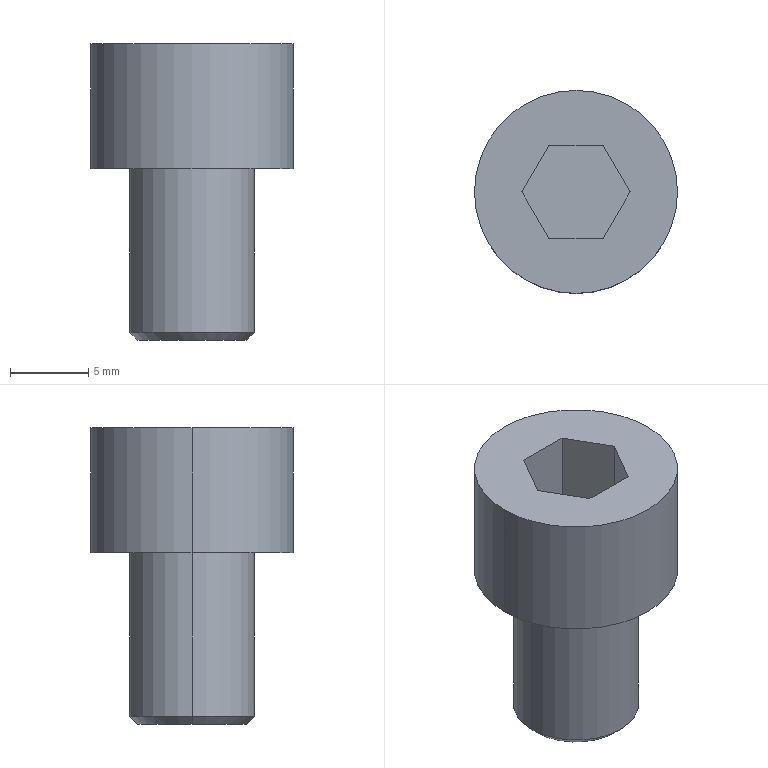Part | Creo | 1 solid | 16 faces | box 13 x 13 x 19 mm | volume 1447 mm3 | plane 10 | cylinder 4 | cone 2 | commonest cylinder face diameters 8 x2 13 x2
STEP:
#1=CARTESIAN_POINT('',(0.,0.,0.));
#2=DIRECTION('',(0.,0.,1.));
#3=DIRECTION('',(1.,0.,0.));
#4=AXIS2_PLACEMENT_3D('',#1,#2,#3);
#5=CARTESIAN_POINT('',(372.601,232.373,-47.934));
#6=VERTEX_POINT('',#5);
#7=CARTESIAN_POINT('',(380.601,232.373,-47.934));
#8=VERTEX_POINT('',#7);
#9=CARTESIAN_POINT('',(376.601,232.373,-47.934));
#10=DIRECTION('',(0.,0.,-1.));
#11=DIRECTION('',(-1.,0.,0.));
#12=AXIS2_PLACEMENT_3D('',#9,#10,#11);
#13=CIRCLE('',#12,4.);
#14=EDGE_CURVE('',#6,#8,#13,.T.);
#15=ORIENTED_EDGE('',*,*,#14,.T.);
#16=CARTESIAN_POINT('',(380.601,232.373,-37.441));
#17=VERTEX_POINT('',#16);
#18=CARTESIAN_POINT('',(380.601,232.373,-37.441));
#19=DIRECTION('',(0.,0.,-1.));
#20=VECTOR('',#19,10.493);
#21=LINE('',#18,#20);
#22=EDGE_CURVE('',#17,#8,#21,.T.);
#23=ORIENTED_EDGE('',*,*,#22,.F.);
#24=CARTESIAN_POINT('',(372.601,232.373,-37.441));
#25=VERTEX_POINT('',#24);
#26=CARTESIAN_POINT('',(376.601,232.373,-37.441));
#27=DIRECTION('',(0.,0.,1.));
#28=DIRECTION('',(1.,0.,0.));
#29=AXIS2_PLACEMENT_3D('',#26,#27,#28);
#30=CIRCLE('',#29,4.);
#31=EDGE_CURVE('',#17,#25,#30,.T.);
#32=ORIENTED_EDGE('',*,*,#31,.T.);
#33=CARTESIAN_POINT('',(372.601,232.373,-37.441));
#34=DIRECTION('',(0.,0.,-1.));
#35=VECTOR('',#34,10.493);
#36=LINE('',#33,#35);
#37=EDGE_CURVE('',#25,#6,#36,.T.);
#38=ORIENTED_EDGE('',*,*,#37,.T.);
#39=EDGE_LOOP('',(#15,#23,#32,#38));
#40=FACE_OUTER_BOUND('',#39,.F.);
#41=CARTESIAN_POINT('',(376.601,232.373,-37.441));
#42=DIRECTION('',(0.,0.,-1.));
#43=DIRECTION('',(-1.,0.,0.));
#44=AXIS2_PLACEMENT_3D('',#41,#42,#43);
#45=CYLINDRICAL_SURFACE('',#44,4.);
#46=ADVANCED_FACE('',(#40),#45,.T.);
#47=CARTESIAN_POINT('',(373.108,232.373,-48.441));
#48=VERTEX_POINT('',#47);
#49=CARTESIAN_POINT('',(380.093,232.373,-48.441));
#50=VERTEX_POINT('',#49);
#51=CARTESIAN_POINT('',(376.601,232.373,-48.441));
#52=DIRECTION('',(0.,0.,-1.));
#53=DIRECTION('',(-1.,0.,0.));
#54=AXIS2_PLACEMENT_3D('',#51,#52,#53);
#55=CIRCLE('',#54,3.493);
#56=EDGE_CURVE('',#48,#50,#55,.T.);
#57=ORIENTED_EDGE('',*,*,#56,.T.);
#58=CARTESIAN_POINT('',(380.093,232.373,-48.441));
#59=DIRECTION('',(0.7071,0.,0.7071));
#60=VECTOR('',#59,0.7176);
#61=LINE('',#58,#60);
#62=EDGE_CURVE('',#50,#8,#61,.T.);
#63=ORIENTED_EDGE('',*,*,#62,.T.);
#64=ORIENTED_EDGE('',*,*,#14,.F.);
#65=CARTESIAN_POINT('',(373.108,232.373,-48.441));
#66=DIRECTION('',(-0.7071,0.,0.7071));
#67=VECTOR('',#66,0.7176);
#68=LINE('',#65,#67);
#69=EDGE_CURVE('',#48,#6,#68,.T.);
#70=ORIENTED_EDGE('',*,*,#69,.F.);
#71=EDGE_LOOP('',(#57,#63,#64,#70));
#72=FACE_OUTER_BOUND('',#71,.F.);
#73=CARTESIAN_POINT('',(376.601,232.373,-48.188));
#74=DIRECTION('',(0.,0.,1.));
#75=DIRECTION('',(1.,0.,0.));
#76=AXIS2_PLACEMENT_3D('',#73,#74,#75);
#77=CONICAL_SURFACE('',#76,3.746,45.);
#78=ADVANCED_FACE('',(#72),#77,.T.);
#79=ORIENTED_EDGE('',*,*,#56,.F.);
#80=CARTESIAN_POINT('',(376.601,232.373,-48.441));
#81=DIRECTION('',(0.,0.,-1.));
#82=DIRECTION('',(1.,0.,0.));
#83=AXIS2_PLACEMENT_3D('',#80,#81,#82);
#84=CIRCLE('',#83,3.493);
#85=EDGE_CURVE('',#50,#48,#84,.T.);
#86=ORIENTED_EDGE('',*,*,#85,.F.);
#87=EDGE_LOOP('',(#79,#86));
#88=FACE_OUTER_BOUND('',#87,.F.);
#89=CARTESIAN_POINT('',(376.601,232.373,-48.441));
#90=DIRECTION('',(0.,0.,1.));
#91=DIRECTION('',(1.,0.,0.));
#92=AXIS2_PLACEMENT_3D('',#89,#90,#91);
#93=PLANE('',#92);
#94=ADVANCED_FACE('',(#88),#93,.F.);
#95=ORIENTED_EDGE('',*,*,#85,.T.);
#96=ORIENTED_EDGE('',*,*,#69,.T.);
#97=CARTESIAN_POINT('',(376.601,232.373,-47.934));
#98=DIRECTION('',(0.,0.,-1.));
#99=DIRECTION('',(1.,0.,0.));
#100=AXIS2_PLACEMENT_3D('',#97,#98,#99);
#101=CIRCLE('',#100,4.);
#102=EDGE_CURVE('',#8,#6,#101,.T.);
#103=ORIENTED_EDGE('',*,*,#102,.F.);
#104=ORIENTED_EDGE('',*,*,#62,.F.);
#105=EDGE_LOOP('',(#95,#96,#103,#104));
#106=FACE_OUTER_BOUND('',#105,.F.);
#107=CARTESIAN_POINT('',(376.601,232.373,-48.188));
#108=DIRECTION('',(0.,0.,1.));
#109=DIRECTION('',(1.,0.,0.));
#110=AXIS2_PLACEMENT_3D('',#107,#108,#109);
#111=CONICAL_SURFACE('',#110,3.746,45.);
#112=ADVANCED_FACE('',(#106),#111,.T.);
#113=ORIENTED_EDGE('',*,*,#102,.T.);
#114=ORIENTED_EDGE('',*,*,#37,.F.);
#115=CARTESIAN_POINT('',(376.601,232.373,-37.441));
#116=DIRECTION('',(0.,0.,1.));
#117=DIRECTION('',(-1.,0.,0.));
#118=AXIS2_PLACEMENT_3D('',#115,#116,#117);
#119=CIRCLE('',#118,4.);
#120=EDGE_CURVE('',#25,#17,#119,.T.);
#121=ORIENTED_EDGE('',*,*,#120,.T.);
#122=ORIENTED_EDGE('',*,*,#22,.T.);
#123=EDGE_LOOP('',(#113,#114,#121,#122));
#124=FACE_OUTER_BOUND('',#123,.F.);
#125=CARTESIAN_POINT('',(376.601,232.373,-37.441));
#126=DIRECTION('',(0.,0.,-1.));
#127=DIRECTION('',(-1.,0.,0.));
#128=AXIS2_PLACEMENT_3D('',#125,#126,#127);
#129=CYLINDRICAL_SURFACE('',#128,4.);
#130=ADVANCED_FACE('',(#124),#129,.T.);
#131=CARTESIAN_POINT('',(370.101,232.373,-37.441));
#132=VERTEX_POINT('',#131);
#133=CARTESIAN_POINT('',(383.101,232.373,-37.441));
#134=VERTEX_POINT('',#133);
#135=CARTESIAN_POINT('',(376.601,232.373,-37.441));
#136=DIRECTION('',(0.,0.,-1.));
#137=DIRECTION('',(-1.,0.,0.));
#138=AXIS2_PLACEMENT_3D('',#135,#136,#137);
#139=CIRCLE('',#138,6.5);
#140=EDGE_CURVE('',#132,#134,#139,.T.);
#141=ORIENTED_EDGE('',*,*,#140,.F.);
#142=CARTESIAN_POINT('',(376.601,232.373,-37.441));
#143=DIRECTION('',(0.,0.,-1.));
#144=DIRECTION('',(1.,0.,0.));
#145=AXIS2_PLACEMENT_3D('',#142,#143,#144);
#146=CIRCLE('',#145,6.5);
#147=EDGE_CURVE('',#134,#132,#146,.T.);
#148=ORIENTED_EDGE('',*,*,#147,.F.);
#149=EDGE_LOOP('',(#141,#148));
#150=FACE_OUTER_BOUND('',#149,.F.);
#151=ORIENTED_EDGE('',*,*,#120,.F.);
#152=ORIENTED_EDGE('',*,*,#31,.F.);
#153=EDGE_LOOP('',(#151,#152));
#154=FACE_BOUND('',#153,.F.);
#155=CARTESIAN_POINT('',(376.601,232.373,-37.441));
#156=DIRECTION('',(0.,0.,-1.));
#157=DIRECTION('',(-1.,0.,0.));
#158=AXIS2_PLACEMENT_3D('',#155,#156,#157);
#159=PLANE('',#158);
#160=ADVANCED_FACE('',(#150,#154),#159,.T.);
#161=CARTESIAN_POINT('',(383.101,232.373,-29.441));
#162=VERTEX_POINT('',#161);
#163=CARTESIAN_POINT('',(370.101,232.373,-29.441));
#164=VERTEX_POINT('',#163);
#165=CARTESIAN_POINT('',(376.601,232.373,-29.441));
#166=DIRECTION('',(0.,0.,1.));
#167=DIRECTION('',(1.,0.,0.));
#168=AXIS2_PLACEMENT_3D('',#165,#166,#167);
#169=CIRCLE('',#168,6.5);
#170=EDGE_CURVE('',#162,#164,#169,.T.);
#171=ORIENTED_EDGE('',*,*,#170,.T.);
#172=CARTESIAN_POINT('',(370.101,232.373,-37.441));
#173=DIRECTION('',(0.,0.,1.));
#174=VECTOR('',#173,8.);
#175=LINE('',#172,#174);
#176=EDGE_CURVE('',#132,#164,#175,.T.);
#177=ORIENTED_EDGE('',*,*,#176,.F.);
#178=ORIENTED_EDGE('',*,*,#140,.T.);
#179=CARTESIAN_POINT('',(383.101,232.373,-37.441));
#180=DIRECTION('',(0.,0.,1.));
#181=VECTOR('',#180,8.);
#182=LINE('',#179,#181);
#183=EDGE_CURVE('',#134,#162,#182,.T.);
#184=ORIENTED_EDGE('',*,*,#183,.T.);
#185=EDGE_LOOP('',(#171,#177,#178,#184));
#186=FACE_OUTER_BOUND('',#185,.F.);
#187=CARTESIAN_POINT('',(376.601,232.373,-37.441));
#188=DIRECTION('',(0.,0.,1.));
#189=DIRECTION('',(1.,0.,0.));
#190=AXIS2_PLACEMENT_3D('',#187,#188,#189);
#191=CYLINDRICAL_SURFACE('',#190,6.5);
#192=ADVANCED_FACE('',(#186),#191,.T.);
#193=CARTESIAN_POINT('',(376.601,232.373,-29.441));
#194=DIRECTION('',(0.,0.,1.));
#195=DIRECTION('',(-1.,0.,0.));
#196=AXIS2_PLACEMENT_3D('',#193,#194,#195);
#197=CIRCLE('',#196,6.5);
#198=EDGE_CURVE('',#164,#162,#197,.T.);
#199=ORIENTED_EDGE('',*,*,#198,.F.);
#200=ORIENTED_EDGE('',*,*,#170,.F.);
#201=EDGE_LOOP('',(#199,#200));
#202=FACE_OUTER_BOUND('',#201,.F.);
#203=CARTESIAN_POINT('',(374.869,235.373,-29.441));
#204=VERTEX_POINT('',#203);
#205=CARTESIAN_POINT('',(378.333,235.373,-29.441));
#206=VERTEX_POINT('',#205);
#207=CARTESIAN_POINT('',(374.869,235.373,-29.441));
#208=DIRECTION('',(1.,0.,0.));
#209=VECTOR('',#208,3.464);
#210=LINE('',#207,#209);
#211=EDGE_CURVE('',#204,#206,#210,.T.);
#212=ORIENTED_EDGE('',*,*,#211,.F.);
#213=CARTESIAN_POINT('',(373.137,232.373,-29.441));
#214=VERTEX_POINT('',#213);
#215=CARTESIAN_POINT('',(373.137,232.373,-29.441));
#216=DIRECTION('',(0.5,0.866,0.));
#217=VECTOR('',#216,3.464);
#218=LINE('',#215,#217);
#219=EDGE_CURVE('',#214,#204,#218,.T.);
#220=ORIENTED_EDGE('',*,*,#219,.F.);
#221=CARTESIAN_POINT('',(374.869,229.373,-29.441));
#222=VERTEX_POINT('',#221);
#223=CARTESIAN_POINT('',(374.869,229.373,-29.441));
#224=DIRECTION('',(-0.5,0.866,0.));
#225=VECTOR('',#224,3.464);
#226=LINE('',#223,#225);
#227=EDGE_CURVE('',#222,#214,#226,.T.);
#228=ORIENTED_EDGE('',*,*,#227,.F.);
#229=CARTESIAN_POINT('',(378.333,229.373,-29.441));
#230=VERTEX_POINT('',#229);
#231=CARTESIAN_POINT('',(378.333,229.373,-29.441));
#232=DIRECTION('',(-1.,0.,0.));
#233=VECTOR('',#232,3.464);
#234=LINE('',#231,#233);
#235=EDGE_CURVE('',#230,#222,#234,.T.);
#236=ORIENTED_EDGE('',*,*,#235,.F.);
#237=CARTESIAN_POINT('',(380.065,232.373,-29.441));
#238=VERTEX_POINT('',#237);
#239=CARTESIAN_POINT('',(380.065,232.373,-29.441));
#240=DIRECTION('',(-0.5,-0.866,0.));
#241=VECTOR('',#240,3.464);
#242=LINE('',#239,#241);
#243=EDGE_CURVE('',#238,#230,#242,.T.);
#244=ORIENTED_EDGE('',*,*,#243,.F.);
#245=CARTESIAN_POINT('',(378.333,235.373,-29.441));
#246=DIRECTION('',(0.5,-0.866,0.));
#247=VECTOR('',#246,3.464);
#248=LINE('',#245,#247);
#249=EDGE_CURVE('',#206,#238,#248,.T.);
#250=ORIENTED_EDGE('',*,*,#249,.F.);
#251=EDGE_LOOP('',(#212,#220,#228,#236,#244,#250));
#252=FACE_BOUND('',#251,.F.);
#253=CARTESIAN_POINT('',(376.601,232.373,-29.441));
#254=DIRECTION('',(0.,0.,1.));
#255=DIRECTION('',(1.,0.,0.));
#256=AXIS2_PLACEMENT_3D('',#253,#254,#255);
#257=PLANE('',#256);
#258=ADVANCED_FACE('',(#202,#252),#257,.T.);
#259=ORIENTED_EDGE('',*,*,#211,.T.);
#260=CARTESIAN_POINT('',(378.333,235.373,-34.721));
#261=VERTEX_POINT('',#260);
#262=CARTESIAN_POINT('',(378.333,235.373,-29.441));
#263=DIRECTION('',(0.,0.,-1.));
#264=VECTOR('',#263,5.28);
#265=LINE('',#262,#264);
#266=EDGE_CURVE('',#206,#261,#265,.T.);
#267=ORIENTED_EDGE('',*,*,#266,.T.);
#268=CARTESIAN_POINT('',(374.869,235.373,-34.721));
#269=VERTEX_POINT('',#268);
#270=CARTESIAN_POINT('',(374.869,235.373,-34.721));
#271=DIRECTION('',(1.,0.,0.));
#272=VECTOR('',#271,3.464);
#273=LINE('',#270,#272);
#274=EDGE_CURVE('',#269,#261,#273,.T.);
#275=ORIENTED_EDGE('',*,*,#274,.F.);
#276=CARTESIAN_POINT('',(374.869,235.373,-29.441));
#277=DIRECTION('',(0.,0.,-1.));
#278=VECTOR('',#277,5.28);
#279=LINE('',#276,#278);
#280=EDGE_CURVE('',#204,#269,#279,.T.);
#281=ORIENTED_EDGE('',*,*,#280,.F.);
#282=EDGE_LOOP('',(#259,#267,#275,#281));
#283=FACE_OUTER_BOUND('',#282,.F.);
#284=CARTESIAN_POINT('',(378.333,235.373,-34.721));
#285=DIRECTION('',(0.,1.,0.));
#286=DIRECTION('',(0.,0.,1.));
#287=AXIS2_PLACEMENT_3D('',#284,#285,#286);
#288=PLANE('',#287);
#289=ADVANCED_FACE('',(#283),#288,.F.);
#290=ORIENTED_EDGE('',*,*,#249,.T.);
#291=CARTESIAN_POINT('',(380.065,232.373,-34.721));
#292=VERTEX_POINT('',#291);
#293=CARTESIAN_POINT('',(380.065,232.373,-29.441));
#294=DIRECTION('',(0.,0.,-1.));
#295=VECTOR('',#294,5.28);
#296=LINE('',#293,#295);
#297=EDGE_CURVE('',#238,#292,#296,.T.);
#298=ORIENTED_EDGE('',*,*,#297,.T.);
#299=CARTESIAN_POINT('',(380.065,232.373,-34.721));
#300=DIRECTION('',(-0.5,0.866,0.));
#301=VECTOR('',#300,3.464);
#302=LINE('',#299,#301);
#303=EDGE_CURVE('',#292,#261,#302,.T.);
#304=ORIENTED_EDGE('',*,*,#303,.T.);
#305=ORIENTED_EDGE('',*,*,#266,.F.);
#306=EDGE_LOOP('',(#290,#298,#304,#305));
#307=FACE_OUTER_BOUND('',#306,.F.);
#308=CARTESIAN_POINT('',(380.065,232.373,-34.721));
#309=DIRECTION('',(0.866,0.5,0.));
#310=DIRECTION('',(-0.5,0.866,0.));
#311=AXIS2_PLACEMENT_3D('',#308,#309,#310);
#312=PLANE('',#311);
#313=ADVANCED_FACE('',(#307),#312,.F.);
#314=ORIENTED_EDGE('',*,*,#243,.T.);
#315=CARTESIAN_POINT('',(378.333,229.373,-34.721));
#316=VERTEX_POINT('',#315);
#317=CARTESIAN_POINT('',(378.333,229.373,-29.441));
#318=DIRECTION('',(0.,0.,-1.));
#319=VECTOR('',#318,5.28);
#320=LINE('',#317,#319);
#321=EDGE_CURVE('',#230,#316,#320,.T.);
#322=ORIENTED_EDGE('',*,*,#321,.T.);
#323=CARTESIAN_POINT('',(378.333,229.373,-34.721));
#324=DIRECTION('',(0.5,0.866,0.));
#325=VECTOR('',#324,3.464);
#326=LINE('',#323,#325);
#327=EDGE_CURVE('',#316,#292,#326,.T.);
#328=ORIENTED_EDGE('',*,*,#327,.T.);
#329=ORIENTED_EDGE('',*,*,#297,.F.);
#330=EDGE_LOOP('',(#314,#322,#328,#329));
#331=FACE_OUTER_BOUND('',#330,.F.);
#332=CARTESIAN_POINT('',(378.333,229.373,-34.721));
#333=DIRECTION('',(0.866,-0.5,0.));
#334=DIRECTION('',(0.5,0.866,0.));
#335=AXIS2_PLACEMENT_3D('',#332,#333,#334);
#336=PLANE('',#335);
#337=ADVANCED_FACE('',(#331),#336,.F.);
#338=ORIENTED_EDGE('',*,*,#235,.T.);
#339=CARTESIAN_POINT('',(374.869,229.373,-34.721));
#340=VERTEX_POINT('',#339);
#341=CARTESIAN_POINT('',(374.869,229.373,-29.441));
#342=DIRECTION('',(0.,0.,-1.));
#343=VECTOR('',#342,5.28);
#344=LINE('',#341,#343);
#345=EDGE_CURVE('',#222,#340,#344,.T.);
#346=ORIENTED_EDGE('',*,*,#345,.T.);
#347=CARTESIAN_POINT('',(378.333,229.373,-34.721));
#348=DIRECTION('',(-1.,0.,0.));
#349=VECTOR('',#348,3.464);
#350=LINE('',#347,#349);
#351=EDGE_CURVE('',#316,#340,#350,.T.);
#352=ORIENTED_EDGE('',*,*,#351,.F.);
#353=ORIENTED_EDGE('',*,*,#321,.F.);
#354=EDGE_LOOP('',(#338,#346,#352,#353));
#355=FACE_OUTER_BOUND('',#354,.F.);
#356=CARTESIAN_POINT('',(374.869,229.373,-34.721));
#357=DIRECTION('',(0.,-1.,0.));
#358=DIRECTION('',(0.,0.,-1.));
#359=AXIS2_PLACEMENT_3D('',#356,#357,#358);
#360=PLANE('',#359);
#361=ADVANCED_FACE('',(#355),#360,.F.);
#362=ORIENTED_EDGE('',*,*,#227,.T.);
#363=CARTESIAN_POINT('',(373.137,232.373,-34.721));
#364=VERTEX_POINT('',#363);
#365=CARTESIAN_POINT('',(373.137,232.373,-29.441));
#366=DIRECTION('',(0.,0.,-1.));
#367=VECTOR('',#366,5.28);
#368=LINE('',#365,#367);
#369=EDGE_CURVE('',#214,#364,#368,.T.);
#370=ORIENTED_EDGE('',*,*,#369,.T.);
#371=CARTESIAN_POINT('',(373.137,232.373,-34.721));
#372=DIRECTION('',(0.5,-0.866,0.));
#373=VECTOR('',#372,3.464);
#374=LINE('',#371,#373);
#375=EDGE_CURVE('',#364,#340,#374,.T.);
#376=ORIENTED_EDGE('',*,*,#375,.T.);
#377=ORIENTED_EDGE('',*,*,#345,.F.);
#378=EDGE_LOOP('',(#362,#370,#376,#377));
#379=FACE_OUTER_BOUND('',#378,.F.);
#380=CARTESIAN_POINT('',(373.137,232.373,-34.721));
#381=DIRECTION('',(-0.866,-0.5,0.));
#382=DIRECTION('',(0.5,-0.866,0.));
#383=AXIS2_PLACEMENT_3D('',#380,#381,#382);
#384=PLANE('',#383);
#385=ADVANCED_FACE('',(#379),#384,.F.);
#386=ORIENTED_EDGE('',*,*,#219,.T.);
#387=ORIENTED_EDGE('',*,*,#280,.T.);
#388=CARTESIAN_POINT('',(374.869,235.373,-34.721));
#389=DIRECTION('',(-0.5,-0.866,0.));
#390=VECTOR('',#389,3.464);
#391=LINE('',#388,#390);
#392=EDGE_CURVE('',#269,#364,#391,.T.);
#393=ORIENTED_EDGE('',*,*,#392,.T.);
#394=ORIENTED_EDGE('',*,*,#369,.F.);
#395=EDGE_LOOP('',(#386,#387,#393,#394));
#396=FACE_OUTER_BOUND('',#395,.F.);
#397=CARTESIAN_POINT('',(374.869,235.373,-34.721));
#398=DIRECTION('',(-0.866,0.5,0.));
#399=DIRECTION('',(-0.5,-0.866,0.));
#400=AXIS2_PLACEMENT_3D('',#397,#398,#399);
#401=PLANE('',#400);
#402=ADVANCED_FACE('',(#396),#401,.F.);
#403=ORIENTED_EDGE('',*,*,#274,.T.);
#404=ORIENTED_EDGE('',*,*,#303,.F.);
#405=ORIENTED_EDGE('',*,*,#327,.F.);
#406=ORIENTED_EDGE('',*,*,#351,.T.);
#407=ORIENTED_EDGE('',*,*,#375,.F.);
#408=ORIENTED_EDGE('',*,*,#392,.F.);
#409=EDGE_LOOP('',(#403,#404,#405,#406,#407,#408));
#410=FACE_OUTER_BOUND('',#409,.F.);
#411=CARTESIAN_POINT('',(374.869,235.373,-34.721));
#412=DIRECTION('',(0.,0.,1.));
#413=DIRECTION('',(1.,0.,0.));
#414=AXIS2_PLACEMENT_3D('',#411,#412,#413);
#415=PLANE('',#414);
#416=ADVANCED_FACE('',(#410),#415,.T.);
#417=ORIENTED_EDGE('',*,*,#198,.T.);
#418=ORIENTED_EDGE('',*,*,#183,.F.);
#419=ORIENTED_EDGE('',*,*,#147,.T.);
#420=ORIENTED_EDGE('',*,*,#176,.T.);
#421=EDGE_LOOP('',(#417,#418,#419,#420));
#422=FACE_OUTER_BOUND('',#421,.F.);
#423=CARTESIAN_POINT('',(376.601,232.373,-37.441));
#424=DIRECTION('',(0.,0.,1.));
#425=DIRECTION('',(1.,0.,0.));
#426=AXIS2_PLACEMENT_3D('',#423,#424,#425);
#427=CYLINDRICAL_SURFACE('',#426,6.5);
#428=ADVANCED_FACE('',(#422),#427,.T.);
#429=CLOSED_SHELL('',(#46,#78,#94,#112,#130,#160,#192,#258,#289,#313,#337,#361,#385,#402,#416,#428));
#430=MANIFOLD_SOLID_BREP('',#429);
#431=(LENGTH_UNIT()NAMED_UNIT(*)SI_UNIT(.MILLI.,.METRE.));
#432=UNCERTAINTY_MEASURE_WITH_UNIT(LENGTH_MEASURE(0.002644),#431,'','');
#433=(NAMED_UNIT(*)PLANE_ANGLE_UNIT()SI_UNIT($,.RADIAN.));
#434=PLANE_ANGLE_MEASURE_WITH_UNIT(PLANE_ANGLE_MEASURE(0.01745),#433);
#435=(CONVERSION_BASED_UNIT('DEGREE',#434)NAMED_UNIT(*)PLANE_ANGLE_UNIT());
#436=(NAMED_UNIT(*)SI_UNIT($,.STERADIAN.)SOLID_ANGLE_UNIT());
#437=(GEOMETRIC_REPRESENTATION_CONTEXT(3)GLOBAL_UNCERTAINTY_ASSIGNED_CONTEXT((#432))GLOBAL_UNIT_ASSIGNED_CONTEXT((#431,#435,#436))REPRESENTATION_CONTEXT('',''));
#438=ADVANCED_BREP_SHAPE_REPRESENTATION('',(#4,#430),#437);